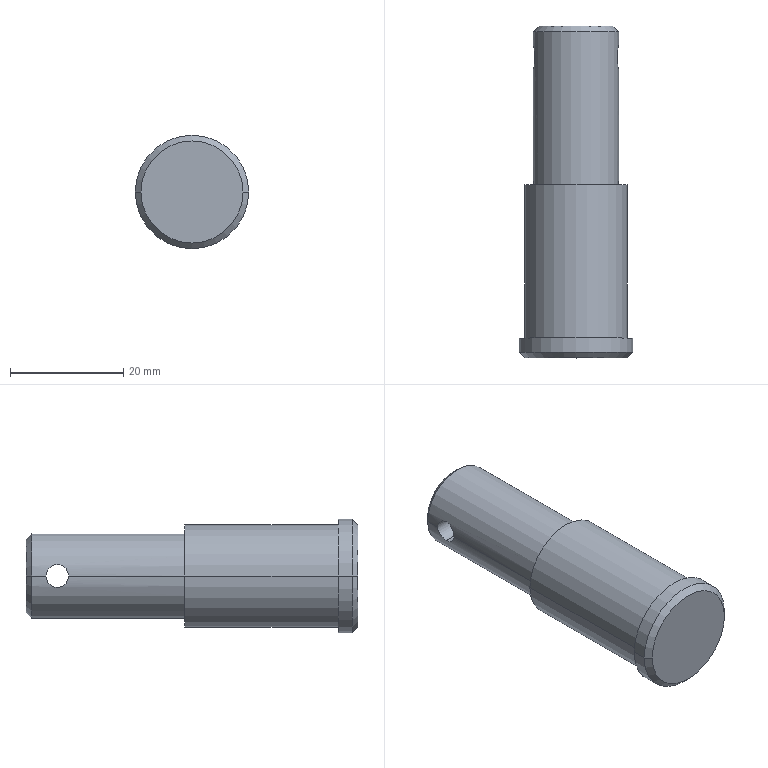Part | SolidWorks | features Chamfer 1, ICE 1, Revolution 1 | 1 solid | 16 faces | box 20 x 58.5 x 20 mm | volume 12679 mm3 | cylinder 8 | cone 4 | plane 4 | commonest cylinder face diameters 4 x2 15 x2 18 x2 20 x2
STEP:
#1=CARTESIAN_POINT('',(9.,-29.25,0.));
#2=VERTEX_POINT('',#1);
#3=CARTESIAN_POINT('',(-9.,-29.25,0.));
#4=VERTEX_POINT('',#3);
#5=CARTESIAN_POINT('',(0.,-29.25,0.));
#6=DIRECTION('',(0.,-1.,0.));
#7=DIRECTION('',(-1.,0.,0.));
#8=AXIS2_PLACEMENT_3D('',#5,#6,#7);
#9=CIRCLE('',#8,9.);
#10=EDGE_CURVE('',#2,#4,#9,.T.);
#11=ORIENTED_EDGE('',*,*,#10,.F.);
#12=CARTESIAN_POINT('',(10.,-28.25,0.));
#13=VERTEX_POINT('',#12);
#14=CARTESIAN_POINT('',(10.,-28.25,0.));
#15=DIRECTION('',(0.7071,0.7071,0.));
#16=VECTOR('',#15,1000.);
#17=LINE('',#14,#16);
#18=EDGE_CURVE('',#2,#13,#17,.T.);
#19=ORIENTED_EDGE('',*,*,#18,.T.);
#20=CARTESIAN_POINT('',(-10.,-28.25,0.));
#21=VERTEX_POINT('',#20);
#22=CARTESIAN_POINT('',(0.,-28.25,0.));
#23=DIRECTION('',(0.,1.,0.));
#24=DIRECTION('',(-1.,0.,0.));
#25=AXIS2_PLACEMENT_3D('',#22,#23,#24);
#26=CIRCLE('',#25,10.);
#27=EDGE_CURVE('',#21,#13,#26,.T.);
#28=ORIENTED_EDGE('',*,*,#27,.F.);
#29=CARTESIAN_POINT('',(-10.,-28.25,0.));
#30=DIRECTION('',(-0.7071,0.7071,0.));
#31=VECTOR('',#30,1000.);
#32=LINE('',#29,#31);
#33=EDGE_CURVE('',#4,#21,#32,.T.);
#34=ORIENTED_EDGE('',*,*,#33,.F.);
#35=EDGE_LOOP('',(#11,#19,#28,#34));
#36=FACE_OUTER_BOUND('',#35,.T.);
#37=CARTESIAN_POINT('',(0.,-28.25,0.));
#38=DIRECTION('',(0.,1.,0.));
#39=DIRECTION('',(-1.,0.,0.));
#40=AXIS2_PLACEMENT_3D('',#37,#38,#39);
#41=CONICAL_SURFACE('',#40,10.,0.7854);
#42=ADVANCED_FACE('',(#36),#41,.T.);
#43=CARTESIAN_POINT('',(-6.5,29.25,0.));
#44=VERTEX_POINT('',#43);
#45=CARTESIAN_POINT('',(6.5,29.25,0.));
#46=VERTEX_POINT('',#45);
#47=CARTESIAN_POINT('',(0.,29.25,0.));
#48=DIRECTION('',(0.,1.,0.));
#49=DIRECTION('',(1.,0.,0.));
#50=AXIS2_PLACEMENT_3D('',#47,#48,#49);
#51=CIRCLE('',#50,6.5);
#52=EDGE_CURVE('',#44,#46,#51,.T.);
#53=ORIENTED_EDGE('',*,*,#52,.F.);
#54=CARTESIAN_POINT('',(-7.5,28.25,0.));
#55=VERTEX_POINT('',#54);
#56=CARTESIAN_POINT('',(-6.5,29.25,0.));
#57=DIRECTION('',(-0.7071,-0.7071,0.));
#58=VECTOR('',#57,1000.);
#59=LINE('',#56,#58);
#60=EDGE_CURVE('',#44,#55,#59,.T.);
#61=ORIENTED_EDGE('',*,*,#60,.T.);
#62=CARTESIAN_POINT('',(7.5,28.25,0.));
#63=VERTEX_POINT('',#62);
#64=CARTESIAN_POINT('',(0.,28.25,0.));
#65=DIRECTION('',(0.,-1.,0.));
#66=DIRECTION('',(1.,0.,0.));
#67=AXIS2_PLACEMENT_3D('',#64,#65,#66);
#68=CIRCLE('',#67,7.5);
#69=EDGE_CURVE('',#63,#55,#68,.T.);
#70=ORIENTED_EDGE('',*,*,#69,.F.);
#71=CARTESIAN_POINT('',(6.5,29.25,0.));
#72=DIRECTION('',(0.7071,-0.7071,0.));
#73=VECTOR('',#72,1000.);
#74=LINE('',#71,#73);
#75=EDGE_CURVE('',#46,#63,#74,.T.);
#76=ORIENTED_EDGE('',*,*,#75,.F.);
#77=EDGE_LOOP('',(#53,#61,#70,#76));
#78=FACE_OUTER_BOUND('',#77,.T.);
#79=CARTESIAN_POINT('',(0.,29.25,0.));
#80=DIRECTION('',(0.,-1.,0.));
#81=DIRECTION('',(1.,0.,0.));
#82=AXIS2_PLACEMENT_3D('',#79,#80,#81);
#83=CONICAL_SURFACE('',#82,6.5,0.7854);
#84=ADVANCED_FACE('',(#78),#83,.T.);
#85=CARTESIAN_POINT('',(-7.228,23.75,2.));
#86=VERTEX_POINT('',#85);
#87=CARTESIAN_POINT('',(-7.5,21.75,0.));
#88=VERTEX_POINT('',#87);
#89=CARTESIAN_POINT('',(-7.228,23.75,2.));
#90=CARTESIAN_POINT('',(-7.228,23.618,2.));
#91=CARTESIAN_POINT('',(-7.232,23.488,1.987));
#92=CARTESIAN_POINT('',(-7.246,23.231,1.936));
#93=CARTESIAN_POINT('',(-7.256,23.103,1.897));
#94=CARTESIAN_POINT('',(-7.294,22.742,1.747));
#95=CARTESIAN_POINT('',(-7.33,22.52,1.598));
#96=CARTESIAN_POINT('',(-7.383,22.245,1.323));
#97=CARTESIAN_POINT('',(-7.401,22.161,1.222));
#98=CARTESIAN_POINT('',(-7.433,22.015,1.004));
#99=CARTESIAN_POINT('',(-7.448,21.954,0.8894));
#100=CARTESIAN_POINT('',(-7.473,21.854,0.6486));
#101=CARTESIAN_POINT('',(-7.483,21.815,0.521));
#102=CARTESIAN_POINT('',(-7.496,21.763,0.2635));
#103=CARTESIAN_POINT('',(-7.5,21.75,0.1327));
#104=CARTESIAN_POINT('',(-7.5,21.75,0.));
#105=B_SPLINE_CURVE_WITH_KNOTS('',3,(#89,#90,#91,#92,#93,#94,#95,#96,#97,#98,#99,#100,#101,#102,#103,#104),.UNSPECIFIED.,.F.,.F.,(4,2,2,2,2,2,2,4),(0.009422,0.009814,0.01021,0.01099,0.01138,0.01178,0.01217,0.01256),.UNSPECIFIED.);
#106=EDGE_CURVE('',#86,#88,#105,.T.);
#107=ORIENTED_EDGE('',*,*,#106,.F.);
#108=CARTESIAN_POINT('',(7.228,23.75,2.));
#109=VERTEX_POINT('',#108);
#110=CARTESIAN_POINT('',(-10.,23.75,2.));
#111=DIRECTION('',(1.,0.,0.));
#112=VECTOR('',#111,1000.);
#113=LINE('',#110,#112);
#114=EDGE_CURVE('',#86,#109,#113,.T.);
#115=ORIENTED_EDGE('',*,*,#114,.T.);
#116=CARTESIAN_POINT('',(7.5,21.75,0.));
#117=VERTEX_POINT('',#116);
#118=CARTESIAN_POINT('',(7.5,21.75,0.));
#119=CARTESIAN_POINT('',(7.5,21.75,0.1311));
#120=CARTESIAN_POINT('',(7.496,21.763,0.2643));
#121=CARTESIAN_POINT('',(7.483,21.815,0.5212));
#122=CARTESIAN_POINT('',(7.473,21.853,0.6462));
#123=CARTESIAN_POINT('',(7.436,22.004,1.01));
#124=CARTESIAN_POINT('',(7.401,22.151,1.23));
#125=CARTESIAN_POINT('',(7.348,22.429,1.507));
#126=CARTESIAN_POINT('',(7.33,22.529,1.59));
#127=CARTESIAN_POINT('',(7.297,22.746,1.734));
#128=CARTESIAN_POINT('',(7.282,22.863,1.797));
#129=CARTESIAN_POINT('',(7.256,23.104,1.897));
#130=CARTESIAN_POINT('',(7.246,23.229,1.935));
#131=CARTESIAN_POINT('',(7.232,23.486,1.987));
#132=CARTESIAN_POINT('',(7.228,23.619,2.));
#133=CARTESIAN_POINT('',(7.228,23.75,2.));
#134=B_SPLINE_CURVE_WITH_KNOTS('',3,(#118,#119,#120,#121,#122,#123,#124,#125,#126,#127,#128,#129,#130,#131,#132,#133),.UNSPECIFIED.,.F.,.F.,(4,2,2,2,2,2,2,4),(0.003142,0.003534,0.003926,0.004711,0.005104,0.005496,0.005889,0.006281),.UNSPECIFIED.);
#135=EDGE_CURVE('',#117,#109,#134,.T.);
#136=ORIENTED_EDGE('',*,*,#135,.F.);
#137=CARTESIAN_POINT('',(7.228,23.75,-2.));
#138=VERTEX_POINT('',#137);
#139=CARTESIAN_POINT('',(7.228,23.75,-2.));
#140=CARTESIAN_POINT('',(7.228,23.617,-2.));
#141=CARTESIAN_POINT('',(7.232,23.487,-1.987));
#142=CARTESIAN_POINT('',(7.246,23.23,-1.936));
#143=CARTESIAN_POINT('',(7.256,23.103,-1.897));
#144=CARTESIAN_POINT('',(7.282,22.861,-1.796));
#145=CARTESIAN_POINT('',(7.297,22.746,-1.735));
#146=CARTESIAN_POINT('',(7.33,22.529,-1.59));
#147=CARTESIAN_POINT('',(7.348,22.427,-1.505));
#148=CARTESIAN_POINT('',(7.401,22.152,-1.23));
#149=CARTESIAN_POINT('',(7.436,22.003,-1.008));
#150=CARTESIAN_POINT('',(7.473,21.853,-0.6467));
#151=CARTESIAN_POINT('',(7.483,21.814,-0.52));
#152=CARTESIAN_POINT('',(7.497,21.763,-0.2614));
#153=CARTESIAN_POINT('',(7.5,21.75,-0.1312));
#154=CARTESIAN_POINT('',(7.5,21.75,0.));
#155=B_SPLINE_CURVE_WITH_KNOTS('',3,(#139,#140,#141,#142,#143,#144,#145,#146,#147,#148,#149,#150,#151,#152,#153,#154),.UNSPECIFIED.,.F.,.F.,(4,2,2,2,2,2,2,4),(0.,0.0003927,0.0007854,0.001178,0.001571,0.002356,0.002749,0.003142),.UNSPECIFIED.);
#156=EDGE_CURVE('',#138,#117,#155,.T.);
#157=ORIENTED_EDGE('',*,*,#156,.F.);
#158=CARTESIAN_POINT('',(-7.228,23.75,-2.));
#159=VERTEX_POINT('',#158);
#160=CARTESIAN_POINT('',(-10.,23.75,-2.));
#161=DIRECTION('',(1.,0.,0.));
#162=VECTOR('',#161,1000.);
#163=LINE('',#160,#162);
#164=EDGE_CURVE('',#159,#138,#163,.T.);
#165=ORIENTED_EDGE('',*,*,#164,.F.);
#166=CARTESIAN_POINT('',(-7.5,21.75,0.));
#167=CARTESIAN_POINT('',(-7.5,21.75,-0.1328));
#168=CARTESIAN_POINT('',(-7.496,21.763,-0.2633));
#169=CARTESIAN_POINT('',(-7.483,21.814,-0.5199));
#170=CARTESIAN_POINT('',(-7.473,21.853,-0.6473));
#171=CARTESIAN_POINT('',(-7.448,21.954,-0.8893));
#172=CARTESIAN_POINT('',(-7.433,22.015,-1.004));
#173=CARTESIAN_POINT('',(-7.401,22.161,-1.221));
#174=CARTESIAN_POINT('',(-7.383,22.245,-1.323));
#175=CARTESIAN_POINT('',(-7.33,22.52,-1.599));
#176=CARTESIAN_POINT('',(-7.294,22.743,-1.747));
#177=CARTESIAN_POINT('',(-7.256,23.103,-1.897));
#178=CARTESIAN_POINT('',(-7.246,23.23,-1.936));
#179=CARTESIAN_POINT('',(-7.232,23.489,-1.987));
#180=CARTESIAN_POINT('',(-7.228,23.619,-2.));
#181=CARTESIAN_POINT('',(-7.228,23.75,-2.));
#182=B_SPLINE_CURVE_WITH_KNOTS('',3,(#166,#167,#168,#169,#170,#171,#172,#173,#174,#175,#176,#177,#178,#179,#180,#181),.UNSPECIFIED.,.F.,.F.,(4,2,2,2,2,2,2,4),(0.,0.0003927,0.0007854,0.001178,0.001571,0.002356,0.002749,0.003142),.UNSPECIFIED.);
#183=EDGE_CURVE('',#88,#159,#182,.T.);
#184=ORIENTED_EDGE('',*,*,#183,.F.);
#185=EDGE_LOOP('',(#107,#115,#136,#157,#165,#184));
#186=FACE_OUTER_BOUND('',#185,.T.);
#187=CARTESIAN_POINT('',(-10.,23.75,0.));
#188=DIRECTION('',(1.,0.,0.));
#189=DIRECTION('',(0.,0.,-1.));
#190=AXIS2_PLACEMENT_3D('',#187,#188,#189);
#191=CYLINDRICAL_SURFACE('',#190,2.);
#192=ADVANCED_FACE('',(#186),#191,.F.);
#193=CARTESIAN_POINT('',(-7.5,1.25,0.));
#194=VERTEX_POINT('',#193);
#195=CARTESIAN_POINT('',(7.5,1.25,0.));
#196=VERTEX_POINT('',#195);
#197=CARTESIAN_POINT('',(0.,1.25,0.));
#198=DIRECTION('',(0.,1.,0.));
#199=DIRECTION('',(-1.,0.,0.));
#200=AXIS2_PLACEMENT_3D('',#197,#198,#199);
#201=CIRCLE('',#200,7.5);
#202=EDGE_CURVE('',#194,#196,#201,.T.);
#203=ORIENTED_EDGE('',*,*,#202,.T.);
#204=CARTESIAN_POINT('',(7.5,29.25,0.));
#205=DIRECTION('',(0.,1.,0.));
#206=VECTOR('',#205,1000.);
#207=LINE('',#204,#206);
#208=EDGE_CURVE('',#196,#117,#207,.T.);
#209=ORIENTED_EDGE('',*,*,#208,.T.);
#210=ORIENTED_EDGE('',*,*,#135,.T.);
#211=CARTESIAN_POINT('',(7.5,25.75,0.));
#212=VERTEX_POINT('',#211);
#213=CARTESIAN_POINT('',(7.228,23.75,2.));
#214=CARTESIAN_POINT('',(7.228,24.012,2.));
#215=CARTESIAN_POINT('',(7.244,24.276,1.947));
#216=CARTESIAN_POINT('',(7.282,24.637,1.797));
#217=CARTESIAN_POINT('',(7.297,24.754,1.734));
#218=CARTESIAN_POINT('',(7.33,24.971,1.589));
#219=CARTESIAN_POINT('',(7.348,25.072,1.507));
#220=CARTESIAN_POINT('',(7.383,25.256,1.322));
#221=CARTESIAN_POINT('',(7.401,25.34,1.22));
#222=CARTESIAN_POINT('',(7.433,25.484,1.004));
#223=CARTESIAN_POINT('',(7.448,25.546,0.8897));
#224=CARTESIAN_POINT('',(7.473,25.647,0.646));
#225=CARTESIAN_POINT('',(7.483,25.686,0.5204));
#226=CARTESIAN_POINT('',(7.496,25.737,0.2642));
#227=CARTESIAN_POINT('',(7.5,25.75,0.1319));
#228=CARTESIAN_POINT('',(7.5,25.75,0.));
#229=B_SPLINE_CURVE_WITH_KNOTS('',3,(#213,#214,#215,#216,#217,#218,#219,#220,#221,#222,#223,#224,#225,#226,#227,#228),.UNSPECIFIED.,.F.,.F.,(4,2,2,2,2,2,2,4),(0.006281,0.007066,0.007459,0.007852,0.008244,0.008637,0.009029,0.009422),.UNSPECIFIED.);
#230=EDGE_CURVE('',#109,#212,#229,.T.);
#231=ORIENTED_EDGE('',*,*,#230,.T.);
#232=CARTESIAN_POINT('',(7.5,29.25,0.));
#233=DIRECTION('',(0.,1.,0.));
#234=VECTOR('',#233,1000.);
#235=LINE('',#232,#234);
#236=EDGE_CURVE('',#212,#63,#235,.T.);
#237=ORIENTED_EDGE('',*,*,#236,.T.);
#238=ORIENTED_EDGE('',*,*,#69,.T.);
#239=CARTESIAN_POINT('',(-7.5,25.75,0.));
#240=VERTEX_POINT('',#239);
#241=CARTESIAN_POINT('',(-7.5,29.25,0.));
#242=DIRECTION('',(0.,1.,0.));
#243=VECTOR('',#242,1000.);
#244=LINE('',#241,#243);
#245=EDGE_CURVE('',#240,#55,#244,.T.);
#246=ORIENTED_EDGE('',*,*,#245,.F.);
#247=CARTESIAN_POINT('',(-7.5,25.75,0.));
#248=CARTESIAN_POINT('',(-7.5,25.75,0.2618));
#249=CARTESIAN_POINT('',(-7.485,25.697,0.5261));
#250=CARTESIAN_POINT('',(-7.448,25.547,0.8875));
#251=CARTESIAN_POINT('',(-7.433,25.484,1.005));
#252=CARTESIAN_POINT('',(-7.401,25.339,1.221));
#253=CARTESIAN_POINT('',(-7.383,25.257,1.322));
#254=CARTESIAN_POINT('',(-7.348,25.072,1.506));
#255=CARTESIAN_POINT('',(-7.33,24.97,1.59));
#256=CARTESIAN_POINT('',(-7.297,24.754,1.734));
#257=CARTESIAN_POINT('',(-7.282,24.64,1.796));
#258=CARTESIAN_POINT('',(-7.256,24.396,1.897));
#259=CARTESIAN_POINT('',(-7.246,24.27,1.936));
#260=CARTESIAN_POINT('',(-7.232,24.014,1.987));
#261=CARTESIAN_POINT('',(-7.228,23.882,2.));
#262=CARTESIAN_POINT('',(-7.228,23.75,2.));
#263=B_SPLINE_CURVE_WITH_KNOTS('',3,(#247,#248,#249,#250,#251,#252,#253,#254,#255,#256,#257,#258,#259,#260,#261,#262),.UNSPECIFIED.,.F.,.F.,(4,2,2,2,2,2,2,4),(0.006281,0.007067,0.007459,0.007852,0.008244,0.008637,0.009029,0.009422),.UNSPECIFIED.);
#264=EDGE_CURVE('',#240,#86,#263,.T.);
#265=ORIENTED_EDGE('',*,*,#264,.T.);
#266=ORIENTED_EDGE('',*,*,#106,.T.);
#267=CARTESIAN_POINT('',(-7.5,29.25,0.));
#268=DIRECTION('',(0.,1.,0.));
#269=VECTOR('',#268,1000.);
#270=LINE('',#267,#269);
#271=EDGE_CURVE('',#194,#88,#270,.T.);
#272=ORIENTED_EDGE('',*,*,#271,.F.);
#273=EDGE_LOOP('',(#203,#209,#210,#231,#237,#238,#246,#265,#266,#272));
#274=FACE_OUTER_BOUND('',#273,.T.);
#275=CARTESIAN_POINT('',(0.,29.25,0.));
#276=DIRECTION('',(0.,1.,0.));
#277=DIRECTION('',(-1.,0.,0.));
#278=AXIS2_PLACEMENT_3D('',#275,#276,#277);
#279=CYLINDRICAL_SURFACE('',#278,7.5);
#280=ADVANCED_FACE('',(#274),#279,.T.);
#281=CARTESIAN_POINT('',(-9.,-25.75,0.));
#282=VERTEX_POINT('',#281);
#283=CARTESIAN_POINT('',(9.,-25.75,0.));
#284=VERTEX_POINT('',#283);
#285=CARTESIAN_POINT('',(0.,-25.75,0.));
#286=DIRECTION('',(0.,1.,0.));
#287=DIRECTION('',(-1.,0.,0.));
#288=AXIS2_PLACEMENT_3D('',#285,#286,#287);
#289=CIRCLE('',#288,9.);
#290=EDGE_CURVE('',#282,#284,#289,.T.);
#291=ORIENTED_EDGE('',*,*,#290,.T.);
#292=CARTESIAN_POINT('',(9.,1.25,0.));
#293=VERTEX_POINT('',#292);
#294=CARTESIAN_POINT('',(9.,29.25,0.));
#295=DIRECTION('',(0.,1.,0.));
#296=VECTOR('',#295,1000.);
#297=LINE('',#294,#296);
#298=EDGE_CURVE('',#284,#293,#297,.T.);
#299=ORIENTED_EDGE('',*,*,#298,.T.);
#300=CARTESIAN_POINT('',(-9.,1.25,0.));
#301=VERTEX_POINT('',#300);
#302=CARTESIAN_POINT('',(0.,1.25,0.));
#303=DIRECTION('',(0.,1.,0.));
#304=DIRECTION('',(-1.,0.,0.));
#305=AXIS2_PLACEMENT_3D('',#302,#303,#304);
#306=CIRCLE('',#305,9.);
#307=EDGE_CURVE('',#301,#293,#306,.T.);
#308=ORIENTED_EDGE('',*,*,#307,.F.);
#309=CARTESIAN_POINT('',(-9.,29.25,0.));
#310=DIRECTION('',(0.,1.,0.));
#311=VECTOR('',#310,1000.);
#312=LINE('',#309,#311);
#313=EDGE_CURVE('',#282,#301,#312,.T.);
#314=ORIENTED_EDGE('',*,*,#313,.F.);
#315=EDGE_LOOP('',(#291,#299,#308,#314));
#316=FACE_OUTER_BOUND('',#315,.T.);
#317=CARTESIAN_POINT('',(0.,29.25,0.));
#318=DIRECTION('',(0.,1.,0.));
#319=DIRECTION('',(-1.,0.,0.));
#320=AXIS2_PLACEMENT_3D('',#317,#318,#319);
#321=CYLINDRICAL_SURFACE('',#320,9.);
#322=ADVANCED_FACE('',(#316),#321,.T.);
#323=ORIENTED_EDGE('',*,*,#27,.T.);
#324=CARTESIAN_POINT('',(10.,-25.75,0.));
#325=VERTEX_POINT('',#324);
#326=CARTESIAN_POINT('',(10.,29.25,0.));
#327=DIRECTION('',(0.,1.,0.));
#328=VECTOR('',#327,1000.);
#329=LINE('',#326,#328);
#330=EDGE_CURVE('',#13,#325,#329,.T.);
#331=ORIENTED_EDGE('',*,*,#330,.T.);
#332=CARTESIAN_POINT('',(-10.,-25.75,0.));
#333=VERTEX_POINT('',#332);
#334=CARTESIAN_POINT('',(0.,-25.75,0.));
#335=DIRECTION('',(0.,1.,0.));
#336=DIRECTION('',(-1.,0.,0.));
#337=AXIS2_PLACEMENT_3D('',#334,#335,#336);
#338=CIRCLE('',#337,10.);
#339=EDGE_CURVE('',#333,#325,#338,.T.);
#340=ORIENTED_EDGE('',*,*,#339,.F.);
#341=CARTESIAN_POINT('',(-10.,29.25,0.));
#342=DIRECTION('',(0.,1.,0.));
#343=VECTOR('',#342,1000.);
#344=LINE('',#341,#343);
#345=EDGE_CURVE('',#21,#333,#344,.T.);
#346=ORIENTED_EDGE('',*,*,#345,.F.);
#347=EDGE_LOOP('',(#323,#331,#340,#346));
#348=FACE_OUTER_BOUND('',#347,.T.);
#349=CARTESIAN_POINT('',(0.,29.25,0.));
#350=DIRECTION('',(0.,1.,0.));
#351=DIRECTION('',(-1.,0.,0.));
#352=AXIS2_PLACEMENT_3D('',#349,#350,#351);
#353=CYLINDRICAL_SURFACE('',#352,10.);
#354=ADVANCED_FACE('',(#348),#353,.T.);
#355=CARTESIAN_POINT('',(0.,-29.25,0.));
#356=DIRECTION('',(0.,-1.,0.));
#357=DIRECTION('',(-1.,0.,0.));
#358=AXIS2_PLACEMENT_3D('',#355,#356,#357);
#359=CIRCLE('',#358,9.);
#360=EDGE_CURVE('',#4,#2,#359,.T.);
#361=ORIENTED_EDGE('',*,*,#360,.T.);
#362=ORIENTED_EDGE('',*,*,#10,.T.);
#363=EDGE_LOOP('',(#361,#362));
#364=FACE_OUTER_BOUND('',#363,.T.);
#365=CARTESIAN_POINT('',(0.,-29.25,0.));
#366=DIRECTION('',(0.,1.,0.));
#367=DIRECTION('',(-1.,0.,0.));
#368=AXIS2_PLACEMENT_3D('',#365,#366,#367);
#369=PLANE('',#368);
#370=ADVANCED_FACE('',(#364),#369,.F.);
#371=ORIENTED_EDGE('',*,*,#330,.F.);
#372=CARTESIAN_POINT('',(0.,-28.25,0.));
#373=DIRECTION('',(0.,1.,0.));
#374=DIRECTION('',(-1.,0.,0.));
#375=AXIS2_PLACEMENT_3D('',#372,#373,#374);
#376=CIRCLE('',#375,10.);
#377=EDGE_CURVE('',#13,#21,#376,.T.);
#378=ORIENTED_EDGE('',*,*,#377,.T.);
#379=ORIENTED_EDGE('',*,*,#345,.T.);
#380=CARTESIAN_POINT('',(0.,-25.75,0.));
#381=DIRECTION('',(0.,1.,0.));
#382=DIRECTION('',(-1.,0.,0.));
#383=AXIS2_PLACEMENT_3D('',#380,#381,#382);
#384=CIRCLE('',#383,10.);
#385=EDGE_CURVE('',#325,#333,#384,.T.);
#386=ORIENTED_EDGE('',*,*,#385,.F.);
#387=EDGE_LOOP('',(#371,#378,#379,#386));
#388=FACE_OUTER_BOUND('',#387,.T.);
#389=CARTESIAN_POINT('',(0.,29.25,0.));
#390=DIRECTION('',(0.,1.,0.));
#391=DIRECTION('',(-1.,0.,0.));
#392=AXIS2_PLACEMENT_3D('',#389,#390,#391);
#393=CYLINDRICAL_SURFACE('',#392,10.);
#394=ADVANCED_FACE('',(#388),#393,.T.);
#395=ORIENTED_EDGE('',*,*,#290,.F.);
#396=CARTESIAN_POINT('',(0.,-25.75,0.));
#397=DIRECTION('',(0.,1.,0.));
#398=DIRECTION('',(-1.,0.,0.));
#399=AXIS2_PLACEMENT_3D('',#396,#397,#398);
#400=CIRCLE('',#399,9.);
#401=EDGE_CURVE('',#284,#282,#400,.T.);
#402=ORIENTED_EDGE('',*,*,#401,.F.);
#403=EDGE_LOOP('',(#395,#402));
#404=FACE_BOUND('',#403,.T.);
#405=ORIENTED_EDGE('',*,*,#339,.T.);
#406=ORIENTED_EDGE('',*,*,#385,.T.);
#407=EDGE_LOOP('',(#405,#406));
#408=FACE_OUTER_BOUND('',#407,.T.);
#409=CARTESIAN_POINT('',(9.,-25.75,0.));
#410=DIRECTION('',(0.,-1.,0.));
#411=DIRECTION('',(1.,0.,0.));
#412=AXIS2_PLACEMENT_3D('',#409,#410,#411);
#413=PLANE('',#412);
#414=ADVANCED_FACE('',(#404,#408),#413,.F.);
#415=ORIENTED_EDGE('',*,*,#298,.F.);
#416=ORIENTED_EDGE('',*,*,#401,.T.);
#417=ORIENTED_EDGE('',*,*,#313,.T.);
#418=CARTESIAN_POINT('',(0.,1.25,0.));
#419=DIRECTION('',(0.,1.,0.));
#420=DIRECTION('',(-1.,0.,0.));
#421=AXIS2_PLACEMENT_3D('',#418,#419,#420);
#422=CIRCLE('',#421,9.);
#423=EDGE_CURVE('',#293,#301,#422,.T.);
#424=ORIENTED_EDGE('',*,*,#423,.F.);
#425=EDGE_LOOP('',(#415,#416,#417,#424));
#426=FACE_OUTER_BOUND('',#425,.T.);
#427=CARTESIAN_POINT('',(0.,29.25,0.));
#428=DIRECTION('',(0.,1.,0.));
#429=DIRECTION('',(-1.,0.,0.));
#430=AXIS2_PLACEMENT_3D('',#427,#428,#429);
#431=CYLINDRICAL_SURFACE('',#430,9.);
#432=ADVANCED_FACE('',(#426),#431,.T.);
#433=ORIENTED_EDGE('',*,*,#202,.F.);
#434=CARTESIAN_POINT('',(0.,1.25,0.));
#435=DIRECTION('',(0.,1.,0.));
#436=DIRECTION('',(-1.,0.,0.));
#437=AXIS2_PLACEMENT_3D('',#434,#435,#436);
#438=CIRCLE('',#437,7.5);
#439=EDGE_CURVE('',#196,#194,#438,.T.);
#440=ORIENTED_EDGE('',*,*,#439,.F.);
#441=EDGE_LOOP('',(#433,#440));
#442=FACE_BOUND('',#441,.T.);
#443=ORIENTED_EDGE('',*,*,#307,.T.);
#444=ORIENTED_EDGE('',*,*,#423,.T.);
#445=EDGE_LOOP('',(#443,#444));
#446=FACE_OUTER_BOUND('',#445,.T.);
#447=CARTESIAN_POINT('',(7.5,1.25,0.));
#448=DIRECTION('',(0.,-1.,0.));
#449=DIRECTION('',(1.,0.,0.));
#450=AXIS2_PLACEMENT_3D('',#447,#448,#449);
#451=PLANE('',#450);
#452=ADVANCED_FACE('',(#442,#446),#451,.F.);
#453=ORIENTED_EDGE('',*,*,#208,.F.);
#454=ORIENTED_EDGE('',*,*,#439,.T.);
#455=ORIENTED_EDGE('',*,*,#271,.T.);
#456=ORIENTED_EDGE('',*,*,#183,.T.);
#457=CARTESIAN_POINT('',(-7.228,23.75,-2.));
#458=CARTESIAN_POINT('',(-7.228,23.881,-2.));
#459=CARTESIAN_POINT('',(-7.232,24.014,-1.987));
#460=CARTESIAN_POINT('',(-7.246,24.271,-1.935));
#461=CARTESIAN_POINT('',(-7.256,24.396,-1.897));
#462=CARTESIAN_POINT('',(-7.295,24.76,-1.746));
#463=CARTESIAN_POINT('',(-7.33,24.98,-1.599));
#464=CARTESIAN_POINT('',(-7.383,25.257,-1.321));
#465=CARTESIAN_POINT('',(-7.401,25.34,-1.221));
#466=CARTESIAN_POINT('',(-7.433,25.484,-1.005));
#467=CARTESIAN_POINT('',(-7.448,25.547,-0.8873));
#468=CARTESIAN_POINT('',(-7.473,25.647,-0.6461));
#469=CARTESIAN_POINT('',(-7.483,25.685,-0.5214));
#470=CARTESIAN_POINT('',(-7.496,25.737,-0.2636));
#471=CARTESIAN_POINT('',(-7.5,25.75,-0.1309));
#472=CARTESIAN_POINT('',(-7.5,25.75,0.));
#473=B_SPLINE_CURVE_WITH_KNOTS('',3,(#457,#458,#459,#460,#461,#462,#463,#464,#465,#466,#467,#468,#469,#470,#471,#472),.UNSPECIFIED.,.F.,.F.,(4,2,2,2,2,2,2,4),(0.003142,0.003534,0.003927,0.004712,0.005104,0.005496,0.005889,0.006281),.UNSPECIFIED.);
#474=EDGE_CURVE('',#159,#240,#473,.T.);
#475=ORIENTED_EDGE('',*,*,#474,.T.);
#476=ORIENTED_EDGE('',*,*,#245,.T.);
#477=CARTESIAN_POINT('',(0.,28.25,0.));
#478=DIRECTION('',(0.,-1.,0.));
#479=DIRECTION('',(1.,0.,0.));
#480=AXIS2_PLACEMENT_3D('',#477,#478,#479);
#481=CIRCLE('',#480,7.5);
#482=EDGE_CURVE('',#55,#63,#481,.T.);
#483=ORIENTED_EDGE('',*,*,#482,.T.);
#484=ORIENTED_EDGE('',*,*,#236,.F.);
#485=CARTESIAN_POINT('',(7.5,25.75,0.));
#486=CARTESIAN_POINT('',(7.5,25.75,-0.1318));
#487=CARTESIAN_POINT('',(7.497,25.737,-0.262));
#488=CARTESIAN_POINT('',(7.483,25.686,-0.5191));
#489=CARTESIAN_POINT('',(7.473,25.647,-0.6468));
#490=CARTESIAN_POINT('',(7.436,25.497,-1.008));
#491=CARTESIAN_POINT('',(7.401,25.348,-1.23));
#492=CARTESIAN_POINT('',(7.348,25.073,-1.506));
#493=CARTESIAN_POINT('',(7.33,24.971,-1.589));
#494=CARTESIAN_POINT('',(7.297,24.754,-1.735));
#495=CARTESIAN_POINT('',(7.282,24.639,-1.796));
#496=CARTESIAN_POINT('',(7.256,24.399,-1.896));
#497=CARTESIAN_POINT('',(7.246,24.271,-1.935));
#498=CARTESIAN_POINT('',(7.232,24.013,-1.987));
#499=CARTESIAN_POINT('',(7.228,23.883,-2.));
#500=CARTESIAN_POINT('',(7.228,23.75,-2.));
#501=B_SPLINE_CURVE_WITH_KNOTS('',3,(#485,#486,#487,#488,#489,#490,#491,#492,#493,#494,#495,#496,#497,#498,#499,#500),.UNSPECIFIED.,.F.,.F.,(4,2,2,2,2,2,2,4),(0.009422,0.009814,0.01021,0.01099,0.01138,0.01178,0.01217,0.01256),.UNSPECIFIED.);
#502=EDGE_CURVE('',#212,#138,#501,.T.);
#503=ORIENTED_EDGE('',*,*,#502,.T.);
#504=ORIENTED_EDGE('',*,*,#156,.T.);
#505=EDGE_LOOP('',(#453,#454,#455,#456,#475,#476,#483,#484,#503,#504));
#506=FACE_OUTER_BOUND('',#505,.T.);
#507=CARTESIAN_POINT('',(0.,29.25,0.));
#508=DIRECTION('',(0.,1.,0.));
#509=DIRECTION('',(-1.,0.,0.));
#510=AXIS2_PLACEMENT_3D('',#507,#508,#509);
#511=CYLINDRICAL_SURFACE('',#510,7.5);
#512=ADVANCED_FACE('',(#506),#511,.T.);
#513=CARTESIAN_POINT('',(0.,29.25,0.));
#514=DIRECTION('',(0.,1.,0.));
#515=DIRECTION('',(1.,0.,0.));
#516=AXIS2_PLACEMENT_3D('',#513,#514,#515);
#517=CIRCLE('',#516,6.5);
#518=EDGE_CURVE('',#46,#44,#517,.T.);
#519=ORIENTED_EDGE('',*,*,#518,.T.);
#520=ORIENTED_EDGE('',*,*,#52,.T.);
#521=EDGE_LOOP('',(#519,#520));
#522=FACE_OUTER_BOUND('',#521,.T.);
#523=CARTESIAN_POINT('',(7.5,29.25,0.));
#524=DIRECTION('',(0.,-1.,0.));
#525=DIRECTION('',(1.,0.,0.));
#526=AXIS2_PLACEMENT_3D('',#523,#524,#525);
#527=PLANE('',#526);
#528=ADVANCED_FACE('',(#522),#527,.F.);
#529=ORIENTED_EDGE('',*,*,#114,.F.);
#530=ORIENTED_EDGE('',*,*,#264,.F.);
#531=ORIENTED_EDGE('',*,*,#474,.F.);
#532=ORIENTED_EDGE('',*,*,#164,.T.);
#533=ORIENTED_EDGE('',*,*,#502,.F.);
#534=ORIENTED_EDGE('',*,*,#230,.F.);
#535=EDGE_LOOP('',(#529,#530,#531,#532,#533,#534));
#536=FACE_OUTER_BOUND('',#535,.T.);
#537=CARTESIAN_POINT('',(-10.,23.75,0.));
#538=DIRECTION('',(1.,0.,0.));
#539=DIRECTION('',(0.,0.,-1.));
#540=AXIS2_PLACEMENT_3D('',#537,#538,#539);
#541=CYLINDRICAL_SURFACE('',#540,2.);
#542=ADVANCED_FACE('',(#536),#541,.F.);
#543=ORIENTED_EDGE('',*,*,#60,.F.);
#544=ORIENTED_EDGE('',*,*,#518,.F.);
#545=ORIENTED_EDGE('',*,*,#75,.T.);
#546=ORIENTED_EDGE('',*,*,#482,.F.);
#547=EDGE_LOOP('',(#543,#544,#545,#546));
#548=FACE_OUTER_BOUND('',#547,.T.);
#549=CARTESIAN_POINT('',(0.,29.25,0.));
#550=DIRECTION('',(0.,-1.,0.));
#551=DIRECTION('',(1.,0.,0.));
#552=AXIS2_PLACEMENT_3D('',#549,#550,#551);
#553=CONICAL_SURFACE('',#552,6.5,0.7854);
#554=ADVANCED_FACE('',(#548),#553,.T.);
#555=ORIENTED_EDGE('',*,*,#18,.F.);
#556=ORIENTED_EDGE('',*,*,#360,.F.);
#557=ORIENTED_EDGE('',*,*,#33,.T.);
#558=ORIENTED_EDGE('',*,*,#377,.F.);
#559=EDGE_LOOP('',(#555,#556,#557,#558));
#560=FACE_OUTER_BOUND('',#559,.T.);
#561=CARTESIAN_POINT('',(0.,-28.25,0.));
#562=DIRECTION('',(0.,1.,0.));
#563=DIRECTION('',(-1.,0.,0.));
#564=AXIS2_PLACEMENT_3D('',#561,#562,#563);
#565=CONICAL_SURFACE('',#564,10.,0.7854);
#566=ADVANCED_FACE('',(#560),#565,.T.);
#567=CLOSED_SHELL('',(#42,#84,#192,#280,#322,#354,#370,#394,#414,#432,#452,#512,#528,#542,#554,#566));
#568=MANIFOLD_SOLID_BREP('',#567);
#569=CARTESIAN_POINT('',(0.,0.,0.));
#570=DIRECTION('',(0.,0.,1.));
#571=DIRECTION('',(1.,0.,0.));
#572=AXIS2_PLACEMENT_3D('',#569,#570,#571);
#573=(LENGTH_UNIT()NAMED_UNIT(*)SI_UNIT(.MILLI.,.METRE.));
#574=UNCERTAINTY_MEASURE_WITH_UNIT(LENGTH_MEASURE(0.00001),#573,'','');
#575=(NAMED_UNIT(*)PLANE_ANGLE_UNIT()SI_UNIT($,.RADIAN.));
#576=(NAMED_UNIT(*)SI_UNIT($,.STERADIAN.)SOLID_ANGLE_UNIT());
#577=(GEOMETRIC_REPRESENTATION_CONTEXT(3)GLOBAL_UNCERTAINTY_ASSIGNED_CONTEXT((#574))GLOBAL_UNIT_ASSIGNED_CONTEXT((#573,#575,#576))REPRESENTATION_CONTEXT('',''));
#578=ADVANCED_BREP_SHAPE_REPRESENTATION('',(#568,#572),#577);